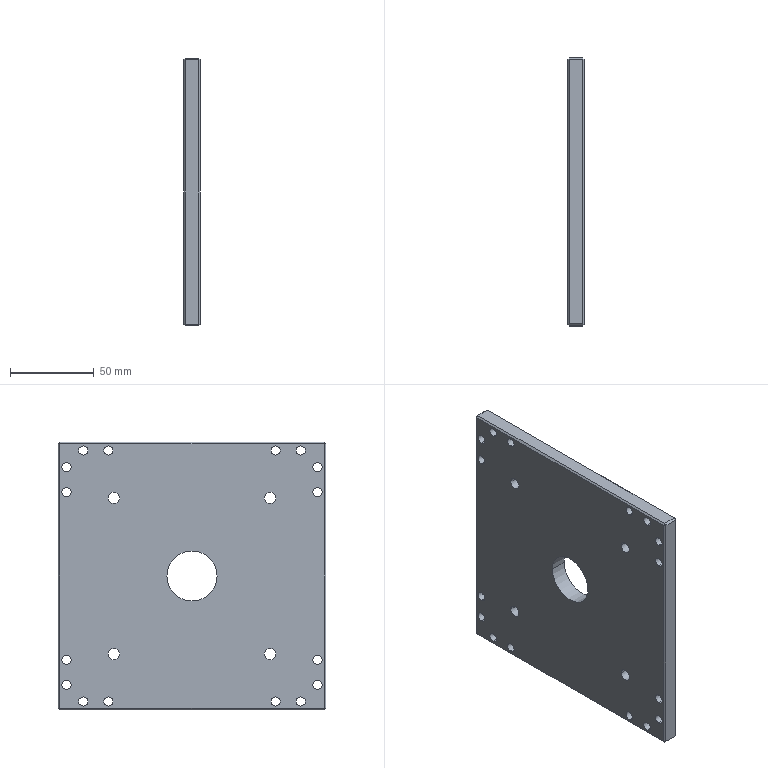Part | STEP file | 05-08 Motor fixing plate | 1 solid | 68 faces | box 10 x 160 x 160 mm | volume 243023 mm3 | cylinder 42 | plane 26 | commonest cylinder face diameters 5.5 x32 6.8 x8 30 x2